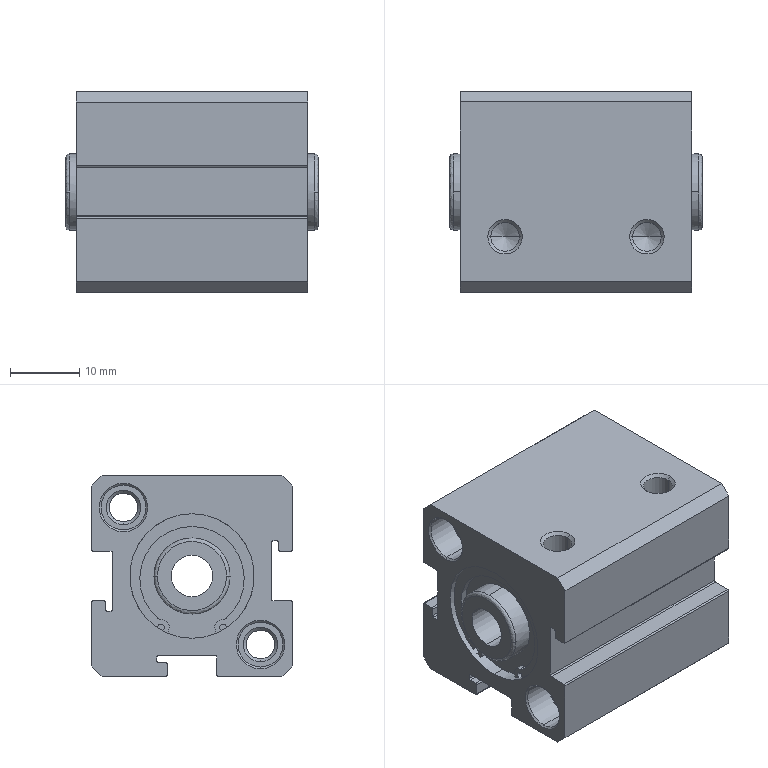Part | SolidWorks | features BaseBody 1 | 1 solid | 142 faces | box 36.5 x 29 x 29 mm | volume 19411 mm3 | cylinder 69 | plane 44 | cone 25 | spline 4 | commonest cylinder face diameters 0.4 x18 1 x12 4.134 x8 6.5 x8 2.4 x6 6 x4